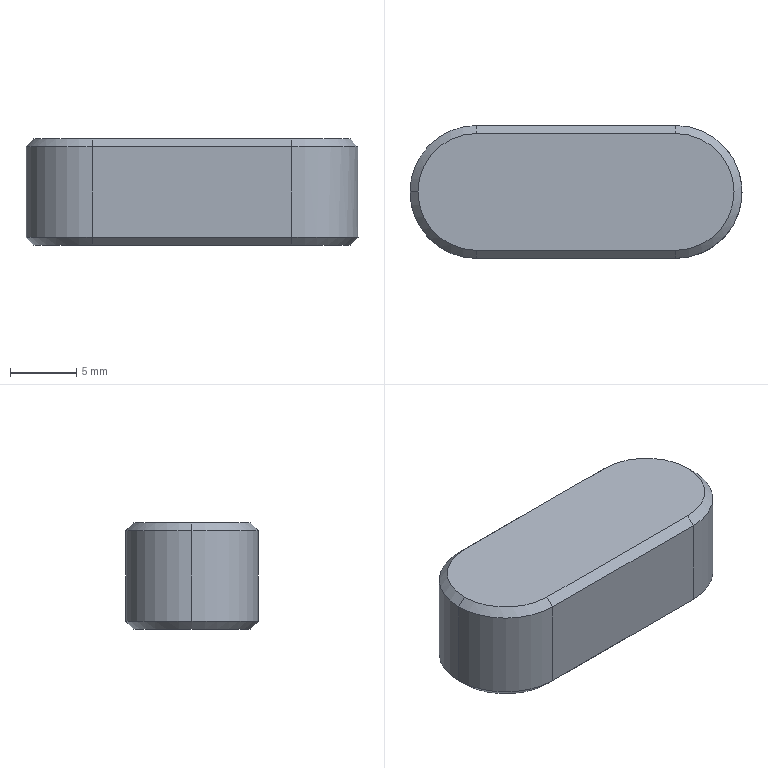Part | SolidWorks | features Boss 2, Chamfer 1, Extrusion 1 | 1 solid | 17 faces | box 25 x 10 x 8 mm | volume 1807 mm3 | plane 8 | cone 6 | cylinder 3 | commonest cylinder face diameters 10 x3
STEP:
#1=CARTESIAN_POINT('',(-19.4,0.,4.));
#2=VERTEX_POINT('',#1);
#3=CARTESIAN_POINT('',(-15.,-4.4,4.));
#4=VERTEX_POINT('',#3);
#5=CARTESIAN_POINT('',(-15.,0.,4.));
#6=DIRECTION('',(0.,0.,1.));
#7=DIRECTION('',(-1.,0.,0.));
#8=AXIS2_PLACEMENT_3D('',#5,#6,#7);
#9=CIRCLE('',#8,4.4);
#10=EDGE_CURVE('',#2,#4,#9,.T.);
#11=ORIENTED_EDGE('',*,*,#10,.F.);
#12=CARTESIAN_POINT('',(-20.,0.,3.4));
#13=VERTEX_POINT('',#12);
#14=CARTESIAN_POINT('',(-19.4,0.,4.));
#15=DIRECTION('',(-0.7071,0.,-0.7071));
#16=VECTOR('',#15,1000.);
#17=LINE('',#14,#16);
#18=EDGE_CURVE('',#2,#13,#17,.T.);
#19=ORIENTED_EDGE('',*,*,#18,.T.);
#20=CARTESIAN_POINT('',(-15.,-5.,3.4));
#21=VERTEX_POINT('',#20);
#22=CARTESIAN_POINT('',(-15.,0.,3.4));
#23=DIRECTION('',(0.,0.,-1.));
#24=DIRECTION('',(-1.,0.,0.));
#25=AXIS2_PLACEMENT_3D('',#22,#23,#24);
#26=CIRCLE('',#25,5.);
#27=EDGE_CURVE('',#21,#13,#26,.T.);
#28=ORIENTED_EDGE('',*,*,#27,.F.);
#29=CARTESIAN_POINT('',(-15.,-4.4,4.));
#30=DIRECTION('',(0.,-0.7071,-0.7071));
#31=VECTOR('',#30,1000.);
#32=LINE('',#29,#31);
#33=EDGE_CURVE('',#4,#21,#32,.T.);
#34=ORIENTED_EDGE('',*,*,#33,.F.);
#35=EDGE_LOOP('',(#11,#19,#28,#34));
#36=FACE_OUTER_BOUND('',#35,.T.);
#37=CARTESIAN_POINT('',(-15.,0.,4.));
#38=DIRECTION('',(0.,0.,-1.));
#39=DIRECTION('',(-1.,0.,0.));
#40=AXIS2_PLACEMENT_3D('',#37,#38,#39);
#41=CONICAL_SURFACE('',#40,4.4,0.7854);
#42=ADVANCED_FACE('',(#36),#41,.T.);
#43=CARTESIAN_POINT('',(4.4,0.,-4.));
#44=VERTEX_POINT('',#43);
#45=CARTESIAN_POINT('',(0.,-4.4,-4.));
#46=VERTEX_POINT('',#45);
#47=CARTESIAN_POINT('',(0.,0.,-4.));
#48=DIRECTION('',(0.,0.,-1.));
#49=DIRECTION('',(-1.,0.,0.));
#50=AXIS2_PLACEMENT_3D('',#47,#48,#49);
#51=CIRCLE('',#50,4.4);
#52=EDGE_CURVE('',#44,#46,#51,.T.);
#53=ORIENTED_EDGE('',*,*,#52,.F.);
#54=CARTESIAN_POINT('',(5.,0.,-3.4));
#55=VERTEX_POINT('',#54);
#56=CARTESIAN_POINT('',(5.,0.,-3.4));
#57=DIRECTION('',(0.7071,0.,0.7071));
#58=VECTOR('',#57,1000.);
#59=LINE('',#56,#58);
#60=EDGE_CURVE('',#44,#55,#59,.T.);
#61=ORIENTED_EDGE('',*,*,#60,.T.);
#62=CARTESIAN_POINT('',(0.,-5.,-3.4));
#63=VERTEX_POINT('',#62);
#64=CARTESIAN_POINT('',(0.,0.,-3.4));
#65=DIRECTION('',(0.,0.,1.));
#66=DIRECTION('',(-1.,0.,0.));
#67=AXIS2_PLACEMENT_3D('',#64,#65,#66);
#68=CIRCLE('',#67,5.);
#69=EDGE_CURVE('',#63,#55,#68,.T.);
#70=ORIENTED_EDGE('',*,*,#69,.F.);
#71=CARTESIAN_POINT('',(0.,-4.4,-4.));
#72=DIRECTION('',(0.,-0.7071,0.7071));
#73=VECTOR('',#72,1000.);
#74=LINE('',#71,#73);
#75=EDGE_CURVE('',#46,#63,#74,.T.);
#76=ORIENTED_EDGE('',*,*,#75,.F.);
#77=EDGE_LOOP('',(#53,#61,#70,#76));
#78=FACE_OUTER_BOUND('',#77,.T.);
#79=CARTESIAN_POINT('',(0.,0.,-3.4));
#80=DIRECTION('',(0.,0.,1.));
#81=DIRECTION('',(1.,0.,0.));
#82=AXIS2_PLACEMENT_3D('',#79,#80,#81);
#83=CONICAL_SURFACE('',#82,5.,0.7854);
#84=ADVANCED_FACE('',(#78),#83,.T.);
#85=ORIENTED_EDGE('',*,*,#27,.T.);
#86=CARTESIAN_POINT('',(-20.,0.,-3.4));
#87=VERTEX_POINT('',#86);
#88=CARTESIAN_POINT('',(-20.,0.,4.));
#89=DIRECTION('',(0.,0.,-1.));
#90=VECTOR('',#89,1000.);
#91=LINE('',#88,#90);
#92=EDGE_CURVE('',#13,#87,#91,.T.);
#93=ORIENTED_EDGE('',*,*,#92,.T.);
#94=CARTESIAN_POINT('',(-15.,-5.,-3.4));
#95=VERTEX_POINT('',#94);
#96=CARTESIAN_POINT('',(-15.,0.,-3.4));
#97=DIRECTION('',(0.,0.,1.));
#98=DIRECTION('',(-1.,0.,0.));
#99=AXIS2_PLACEMENT_3D('',#96,#97,#98);
#100=CIRCLE('',#99,5.);
#101=EDGE_CURVE('',#87,#95,#100,.T.);
#102=ORIENTED_EDGE('',*,*,#101,.T.);
#103=CARTESIAN_POINT('',(-15.,-5.,4.));
#104=DIRECTION('',(0.,0.,-1.));
#105=VECTOR('',#104,1000.);
#106=LINE('',#103,#105);
#107=EDGE_CURVE('',#21,#95,#106,.T.);
#108=ORIENTED_EDGE('',*,*,#107,.F.);
#109=EDGE_LOOP('',(#85,#93,#102,#108));
#110=FACE_OUTER_BOUND('',#109,.T.);
#111=CARTESIAN_POINT('',(-15.,0.,4.));
#112=DIRECTION('',(0.,0.,-1.));
#113=DIRECTION('',(-1.,0.,0.));
#114=AXIS2_PLACEMENT_3D('',#111,#112,#113);
#115=CYLINDRICAL_SURFACE('',#114,5.);
#116=ADVANCED_FACE('',(#110),#115,.T.);
#117=ORIENTED_EDGE('',*,*,#92,.F.);
#118=CARTESIAN_POINT('',(-15.,5.,3.4));
#119=VERTEX_POINT('',#118);
#120=CARTESIAN_POINT('',(-15.,0.,3.4));
#121=DIRECTION('',(0.,0.,-1.));
#122=DIRECTION('',(-1.,0.,0.));
#123=AXIS2_PLACEMENT_3D('',#120,#121,#122);
#124=CIRCLE('',#123,5.);
#125=EDGE_CURVE('',#13,#119,#124,.T.);
#126=ORIENTED_EDGE('',*,*,#125,.T.);
#127=CARTESIAN_POINT('',(-15.,5.,-3.4));
#128=VERTEX_POINT('',#127);
#129=CARTESIAN_POINT('',(-15.,5.,4.));
#130=DIRECTION('',(0.,0.,-1.));
#131=VECTOR('',#130,1000.);
#132=LINE('',#129,#131);
#133=EDGE_CURVE('',#119,#128,#132,.T.);
#134=ORIENTED_EDGE('',*,*,#133,.T.);
#135=CARTESIAN_POINT('',(-15.,0.,-3.4));
#136=DIRECTION('',(0.,0.,1.));
#137=DIRECTION('',(-1.,0.,0.));
#138=AXIS2_PLACEMENT_3D('',#135,#136,#137);
#139=CIRCLE('',#138,5.);
#140=EDGE_CURVE('',#128,#87,#139,.T.);
#141=ORIENTED_EDGE('',*,*,#140,.T.);
#142=EDGE_LOOP('',(#117,#126,#134,#141));
#143=FACE_OUTER_BOUND('',#142,.T.);
#144=CARTESIAN_POINT('',(-15.,0.,4.));
#145=DIRECTION('',(0.,0.,-1.));
#146=DIRECTION('',(-1.,0.,0.));
#147=AXIS2_PLACEMENT_3D('',#144,#145,#146);
#148=CYLINDRICAL_SURFACE('',#147,5.);
#149=ADVANCED_FACE('',(#143),#148,.T.);
#150=ORIENTED_EDGE('',*,*,#107,.T.);
#151=CARTESIAN_POINT('',(0.,-5.,-3.4));
#152=DIRECTION('',(1.,0.,0.));
#153=VECTOR('',#152,1000.);
#154=LINE('',#151,#153);
#155=EDGE_CURVE('',#95,#63,#154,.T.);
#156=ORIENTED_EDGE('',*,*,#155,.T.);
#157=CARTESIAN_POINT('',(0.,-5.,3.4));
#158=VERTEX_POINT('',#157);
#159=CARTESIAN_POINT('',(0.,-5.,4.));
#160=DIRECTION('',(0.,0.,-1.));
#161=VECTOR('',#160,1000.);
#162=LINE('',#159,#161);
#163=EDGE_CURVE('',#158,#63,#162,.T.);
#164=ORIENTED_EDGE('',*,*,#163,.F.);
#165=CARTESIAN_POINT('',(0.,-5.,3.4));
#166=DIRECTION('',(-1.,0.,0.));
#167=VECTOR('',#166,1000.);
#168=LINE('',#165,#167);
#169=EDGE_CURVE('',#158,#21,#168,.T.);
#170=ORIENTED_EDGE('',*,*,#169,.T.);
#171=EDGE_LOOP('',(#150,#156,#164,#170));
#172=FACE_OUTER_BOUND('',#171,.T.);
#173=CARTESIAN_POINT('',(0.,-5.,4.));
#174=DIRECTION('',(0.,1.,0.));
#175=DIRECTION('',(-1.,0.,0.));
#176=AXIS2_PLACEMENT_3D('',#173,#174,#175);
#177=PLANE('',#176);
#178=ADVANCED_FACE('',(#172),#177,.F.);
#179=CARTESIAN_POINT('',(0.,5.,3.4));
#180=VERTEX_POINT('',#179);
#181=CARTESIAN_POINT('',(0.,5.,-3.4));
#182=VERTEX_POINT('',#181);
#183=CARTESIAN_POINT('',(0.,5.,4.));
#184=DIRECTION('',(0.,0.,-1.));
#185=VECTOR('',#184,1000.);
#186=LINE('',#183,#185);
#187=EDGE_CURVE('',#180,#182,#186,.T.);
#188=ORIENTED_EDGE('',*,*,#187,.F.);
#189=CARTESIAN_POINT('',(0.,0.,3.4));
#190=DIRECTION('',(0.,0.,-1.));
#191=DIRECTION('',(-1.,0.,0.));
#192=AXIS2_PLACEMENT_3D('',#189,#190,#191);
#193=CIRCLE('',#192,5.);
#194=EDGE_CURVE('',#180,#158,#193,.T.);
#195=ORIENTED_EDGE('',*,*,#194,.T.);
#196=ORIENTED_EDGE('',*,*,#163,.T.);
#197=ORIENTED_EDGE('',*,*,#69,.T.);
#198=CARTESIAN_POINT('',(0.,0.,-3.4));
#199=DIRECTION('',(0.,0.,1.));
#200=DIRECTION('',(-1.,0.,0.));
#201=AXIS2_PLACEMENT_3D('',#198,#199,#200);
#202=CIRCLE('',#201,5.);
#203=EDGE_CURVE('',#55,#182,#202,.T.);
#204=ORIENTED_EDGE('',*,*,#203,.T.);
#205=EDGE_LOOP('',(#188,#195,#196,#197,#204));
#206=FACE_OUTER_BOUND('',#205,.T.);
#207=CARTESIAN_POINT('',(0.,0.,4.));
#208=DIRECTION('',(0.,0.,-1.));
#209=DIRECTION('',(-1.,0.,0.));
#210=AXIS2_PLACEMENT_3D('',#207,#208,#209);
#211=CYLINDRICAL_SURFACE('',#210,5.);
#212=ADVANCED_FACE('',(#206),#211,.T.);
#213=ORIENTED_EDGE('',*,*,#133,.F.);
#214=CARTESIAN_POINT('',(-15.,5.,3.4));
#215=DIRECTION('',(1.,0.,0.));
#216=VECTOR('',#215,1000.);
#217=LINE('',#214,#216);
#218=EDGE_CURVE('',#119,#180,#217,.T.);
#219=ORIENTED_EDGE('',*,*,#218,.T.);
#220=ORIENTED_EDGE('',*,*,#187,.T.);
#221=CARTESIAN_POINT('',(-15.,5.,-3.4));
#222=DIRECTION('',(-1.,0.,0.));
#223=VECTOR('',#222,1000.);
#224=LINE('',#221,#223);
#225=EDGE_CURVE('',#182,#128,#224,.T.);
#226=ORIENTED_EDGE('',*,*,#225,.T.);
#227=EDGE_LOOP('',(#213,#219,#220,#226));
#228=FACE_OUTER_BOUND('',#227,.T.);
#229=CARTESIAN_POINT('',(-15.,5.,4.));
#230=DIRECTION('',(0.,-1.,0.));
#231=DIRECTION('',(0.,0.,-1.));
#232=AXIS2_PLACEMENT_3D('',#229,#230,#231);
#233=PLANE('',#232);
#234=ADVANCED_FACE('',(#228),#233,.F.);
#235=CARTESIAN_POINT('',(-15.,4.4,4.));
#236=VERTEX_POINT('',#235);
#237=CARTESIAN_POINT('',(-15.,0.,4.));
#238=DIRECTION('',(0.,0.,1.));
#239=DIRECTION('',(-1.,0.,0.));
#240=AXIS2_PLACEMENT_3D('',#237,#238,#239);
#241=CIRCLE('',#240,4.4);
#242=EDGE_CURVE('',#236,#2,#241,.T.);
#243=ORIENTED_EDGE('',*,*,#242,.T.);
#244=ORIENTED_EDGE('',*,*,#10,.T.);
#245=CARTESIAN_POINT('',(0.,-4.4,4.));
#246=VERTEX_POINT('',#245);
#247=CARTESIAN_POINT('',(-15.,-4.4,4.));
#248=DIRECTION('',(1.,0.,0.));
#249=VECTOR('',#248,1000.);
#250=LINE('',#247,#249);
#251=EDGE_CURVE('',#4,#246,#250,.T.);
#252=ORIENTED_EDGE('',*,*,#251,.T.);
#253=CARTESIAN_POINT('',(0.,4.4,4.));
#254=VERTEX_POINT('',#253);
#255=CARTESIAN_POINT('',(0.,0.,4.));
#256=DIRECTION('',(0.,0.,1.));
#257=DIRECTION('',(-1.,0.,0.));
#258=AXIS2_PLACEMENT_3D('',#255,#256,#257);
#259=CIRCLE('',#258,4.4);
#260=EDGE_CURVE('',#246,#254,#259,.T.);
#261=ORIENTED_EDGE('',*,*,#260,.T.);
#262=CARTESIAN_POINT('',(-15.,4.4,4.));
#263=DIRECTION('',(-1.,0.,0.));
#264=VECTOR('',#263,1000.);
#265=LINE('',#262,#264);
#266=EDGE_CURVE('',#254,#236,#265,.T.);
#267=ORIENTED_EDGE('',*,*,#266,.T.);
#268=EDGE_LOOP('',(#243,#244,#252,#261,#267));
#269=FACE_OUTER_BOUND('',#268,.T.);
#270=CARTESIAN_POINT('',(-15.,0.,4.));
#271=DIRECTION('',(0.,0.,-1.));
#272=DIRECTION('',(-1.,0.,0.));
#273=AXIS2_PLACEMENT_3D('',#270,#271,#272);
#274=PLANE('',#273);
#275=ADVANCED_FACE('',(#269),#274,.F.);
#276=CARTESIAN_POINT('',(0.,4.4,-4.));
#277=VERTEX_POINT('',#276);
#278=CARTESIAN_POINT('',(0.,0.,-4.));
#279=DIRECTION('',(0.,0.,-1.));
#280=DIRECTION('',(-1.,0.,0.));
#281=AXIS2_PLACEMENT_3D('',#278,#279,#280);
#282=CIRCLE('',#281,4.4);
#283=EDGE_CURVE('',#277,#44,#282,.T.);
#284=ORIENTED_EDGE('',*,*,#283,.T.);
#285=ORIENTED_EDGE('',*,*,#52,.T.);
#286=CARTESIAN_POINT('',(-15.,-4.4,-4.));
#287=VERTEX_POINT('',#286);
#288=CARTESIAN_POINT('',(-15.,-4.4,-4.));
#289=DIRECTION('',(-1.,0.,0.));
#290=VECTOR('',#289,1000.);
#291=LINE('',#288,#290);
#292=EDGE_CURVE('',#46,#287,#291,.T.);
#293=ORIENTED_EDGE('',*,*,#292,.T.);
#294=CARTESIAN_POINT('',(-15.,4.4,-4.));
#295=VERTEX_POINT('',#294);
#296=CARTESIAN_POINT('',(-15.,0.,-4.));
#297=DIRECTION('',(0.,0.,-1.));
#298=DIRECTION('',(-1.,0.,0.));
#299=AXIS2_PLACEMENT_3D('',#296,#297,#298);
#300=CIRCLE('',#299,4.4);
#301=EDGE_CURVE('',#287,#295,#300,.T.);
#302=ORIENTED_EDGE('',*,*,#301,.T.);
#303=CARTESIAN_POINT('',(0.,4.4,-4.));
#304=DIRECTION('',(1.,0.,0.));
#305=VECTOR('',#304,1000.);
#306=LINE('',#303,#305);
#307=EDGE_CURVE('',#295,#277,#306,.T.);
#308=ORIENTED_EDGE('',*,*,#307,.T.);
#309=EDGE_LOOP('',(#284,#285,#293,#302,#308));
#310=FACE_OUTER_BOUND('',#309,.T.);
#311=CARTESIAN_POINT('',(-15.,0.,-4.));
#312=DIRECTION('',(0.,0.,-1.));
#313=DIRECTION('',(-1.,0.,0.));
#314=AXIS2_PLACEMENT_3D('',#311,#312,#313);
#315=PLANE('',#314);
#316=ADVANCED_FACE('',(#310),#315,.T.);
#317=CARTESIAN_POINT('',(0.,4.4,-4.));
#318=DIRECTION('',(0.,0.7071,0.7071));
#319=VECTOR('',#318,1000.);
#320=LINE('',#317,#319);
#321=EDGE_CURVE('',#277,#182,#320,.T.);
#322=ORIENTED_EDGE('',*,*,#321,.F.);
#323=ORIENTED_EDGE('',*,*,#307,.F.);
#324=CARTESIAN_POINT('',(-15.,5.,-3.4));
#325=DIRECTION('',(0.,-0.7071,-0.7071));
#326=VECTOR('',#325,1000.);
#327=LINE('',#324,#326);
#328=EDGE_CURVE('',#128,#295,#327,.T.);
#329=ORIENTED_EDGE('',*,*,#328,.F.);
#330=ORIENTED_EDGE('',*,*,#225,.F.);
#331=EDGE_LOOP('',(#322,#323,#329,#330));
#332=FACE_OUTER_BOUND('',#331,.T.);
#333=CARTESIAN_POINT('',(-15.,5.,-3.4));
#334=DIRECTION('',(0.,0.7071,-0.7071));
#335=DIRECTION('',(0.,0.7071,0.7071));
#336=AXIS2_PLACEMENT_3D('',#333,#334,#335);
#337=PLANE('',#336);
#338=ADVANCED_FACE('',(#332),#337,.T.);
#339=ORIENTED_EDGE('',*,*,#328,.T.);
#340=ORIENTED_EDGE('',*,*,#301,.F.);
#341=CARTESIAN_POINT('',(-15.,-5.,-3.4));
#342=DIRECTION('',(0.,0.7071,-0.7071));
#343=VECTOR('',#342,1000.);
#344=LINE('',#341,#343);
#345=EDGE_CURVE('',#95,#287,#344,.T.);
#346=ORIENTED_EDGE('',*,*,#345,.F.);
#347=ORIENTED_EDGE('',*,*,#101,.F.);
#348=ORIENTED_EDGE('',*,*,#140,.F.);
#349=EDGE_LOOP('',(#339,#340,#346,#347,#348));
#350=FACE_OUTER_BOUND('',#349,.T.);
#351=CARTESIAN_POINT('',(-15.,0.,-3.4));
#352=DIRECTION('',(0.,0.,1.));
#353=DIRECTION('',(1.,0.,0.));
#354=AXIS2_PLACEMENT_3D('',#351,#352,#353);
#355=CONICAL_SURFACE('',#354,5.,0.7854);
#356=ADVANCED_FACE('',(#350),#355,.T.);
#357=ORIENTED_EDGE('',*,*,#60,.F.);
#358=ORIENTED_EDGE('',*,*,#283,.F.);
#359=ORIENTED_EDGE('',*,*,#321,.T.);
#360=ORIENTED_EDGE('',*,*,#203,.F.);
#361=EDGE_LOOP('',(#357,#358,#359,#360));
#362=FACE_OUTER_BOUND('',#361,.T.);
#363=CARTESIAN_POINT('',(0.,0.,-3.4));
#364=DIRECTION('',(0.,0.,1.));
#365=DIRECTION('',(1.,0.,0.));
#366=AXIS2_PLACEMENT_3D('',#363,#364,#365);
#367=CONICAL_SURFACE('',#366,5.,0.7854);
#368=ADVANCED_FACE('',(#362),#367,.T.);
#369=ORIENTED_EDGE('',*,*,#345,.T.);
#370=ORIENTED_EDGE('',*,*,#292,.F.);
#371=ORIENTED_EDGE('',*,*,#75,.T.);
#372=ORIENTED_EDGE('',*,*,#155,.F.);
#373=EDGE_LOOP('',(#369,#370,#371,#372));
#374=FACE_OUTER_BOUND('',#373,.T.);
#375=CARTESIAN_POINT('',(0.,-5.,-3.4));
#376=DIRECTION('',(0.,-0.7071,-0.7071));
#377=DIRECTION('',(0.,0.7071,-0.7071));
#378=AXIS2_PLACEMENT_3D('',#375,#376,#377);
#379=PLANE('',#378);
#380=ADVANCED_FACE('',(#374),#379,.T.);
#381=CARTESIAN_POINT('',(0.,5.,3.4));
#382=DIRECTION('',(0.,-0.7071,0.7071));
#383=VECTOR('',#382,1000.);
#384=LINE('',#381,#383);
#385=EDGE_CURVE('',#180,#254,#384,.T.);
#386=ORIENTED_EDGE('',*,*,#385,.F.);
#387=ORIENTED_EDGE('',*,*,#218,.F.);
#388=CARTESIAN_POINT('',(-15.,4.4,4.));
#389=DIRECTION('',(0.,0.7071,-0.7071));
#390=VECTOR('',#389,1000.);
#391=LINE('',#388,#390);
#392=EDGE_CURVE('',#236,#119,#391,.T.);
#393=ORIENTED_EDGE('',*,*,#392,.F.);
#394=ORIENTED_EDGE('',*,*,#266,.F.);
#395=EDGE_LOOP('',(#386,#387,#393,#394));
#396=FACE_OUTER_BOUND('',#395,.T.);
#397=CARTESIAN_POINT('',(-15.,4.4,4.));
#398=DIRECTION('',(0.,-0.7071,-0.7071));
#399=DIRECTION('',(0.,0.7071,-0.7071));
#400=AXIS2_PLACEMENT_3D('',#397,#398,#399);
#401=PLANE('',#400);
#402=ADVANCED_FACE('',(#396),#401,.F.);
#403=ORIENTED_EDGE('',*,*,#18,.F.);
#404=ORIENTED_EDGE('',*,*,#242,.F.);
#405=ORIENTED_EDGE('',*,*,#392,.T.);
#406=ORIENTED_EDGE('',*,*,#125,.F.);
#407=EDGE_LOOP('',(#403,#404,#405,#406));
#408=FACE_OUTER_BOUND('',#407,.T.);
#409=CARTESIAN_POINT('',(-15.,0.,4.));
#410=DIRECTION('',(0.,0.,-1.));
#411=DIRECTION('',(-1.,0.,0.));
#412=AXIS2_PLACEMENT_3D('',#409,#410,#411);
#413=CONICAL_SURFACE('',#412,4.4,0.7854);
#414=ADVANCED_FACE('',(#408),#413,.T.);
#415=ORIENTED_EDGE('',*,*,#385,.T.);
#416=ORIENTED_EDGE('',*,*,#260,.F.);
#417=CARTESIAN_POINT('',(0.,-5.,3.4));
#418=DIRECTION('',(0.,0.7071,0.7071));
#419=VECTOR('',#418,1000.);
#420=LINE('',#417,#419);
#421=EDGE_CURVE('',#158,#246,#420,.T.);
#422=ORIENTED_EDGE('',*,*,#421,.F.);
#423=ORIENTED_EDGE('',*,*,#194,.F.);
#424=EDGE_LOOP('',(#415,#416,#422,#423));
#425=FACE_OUTER_BOUND('',#424,.T.);
#426=CARTESIAN_POINT('',(0.,0.,4.));
#427=DIRECTION('',(0.,0.,-1.));
#428=DIRECTION('',(-1.,0.,0.));
#429=AXIS2_PLACEMENT_3D('',#426,#427,#428);
#430=CONICAL_SURFACE('',#429,4.4,0.7854);
#431=ADVANCED_FACE('',(#425),#430,.T.);
#432=ORIENTED_EDGE('',*,*,#33,.T.);
#433=ORIENTED_EDGE('',*,*,#169,.F.);
#434=ORIENTED_EDGE('',*,*,#421,.T.);
#435=ORIENTED_EDGE('',*,*,#251,.F.);
#436=EDGE_LOOP('',(#432,#433,#434,#435));
#437=FACE_OUTER_BOUND('',#436,.T.);
#438=CARTESIAN_POINT('',(-15.,-4.4,4.));
#439=DIRECTION('',(0.,0.7071,-0.7071));
#440=DIRECTION('',(0.,0.7071,0.7071));
#441=AXIS2_PLACEMENT_3D('',#438,#439,#440);
#442=PLANE('',#441);
#443=ADVANCED_FACE('',(#437),#442,.F.);
#444=CLOSED_SHELL('',(#42,#84,#116,#149,#178,#212,#234,#275,#316,#338,#356,#368,#380,#402,#414,#431,#443));
#445=MANIFOLD_SOLID_BREP('',#444);
#446=CARTESIAN_POINT('',(0.,0.,0.));
#447=DIRECTION('',(0.,0.,1.));
#448=DIRECTION('',(1.,0.,0.));
#449=AXIS2_PLACEMENT_3D('',#446,#447,#448);
#450=(LENGTH_UNIT()NAMED_UNIT(*)SI_UNIT(.MILLI.,.METRE.));
#451=UNCERTAINTY_MEASURE_WITH_UNIT(LENGTH_MEASURE(0.00001),#450,'','');
#452=(NAMED_UNIT(*)PLANE_ANGLE_UNIT()SI_UNIT($,.RADIAN.));
#453=(NAMED_UNIT(*)SI_UNIT($,.STERADIAN.)SOLID_ANGLE_UNIT());
#454=(GEOMETRIC_REPRESENTATION_CONTEXT(3)GLOBAL_UNCERTAINTY_ASSIGNED_CONTEXT((#451))GLOBAL_UNIT_ASSIGNED_CONTEXT((#450,#452,#453))REPRESENTATION_CONTEXT('',''));
#455=ADVANCED_BREP_SHAPE_REPRESENTATION('',(#445,#449),#454);